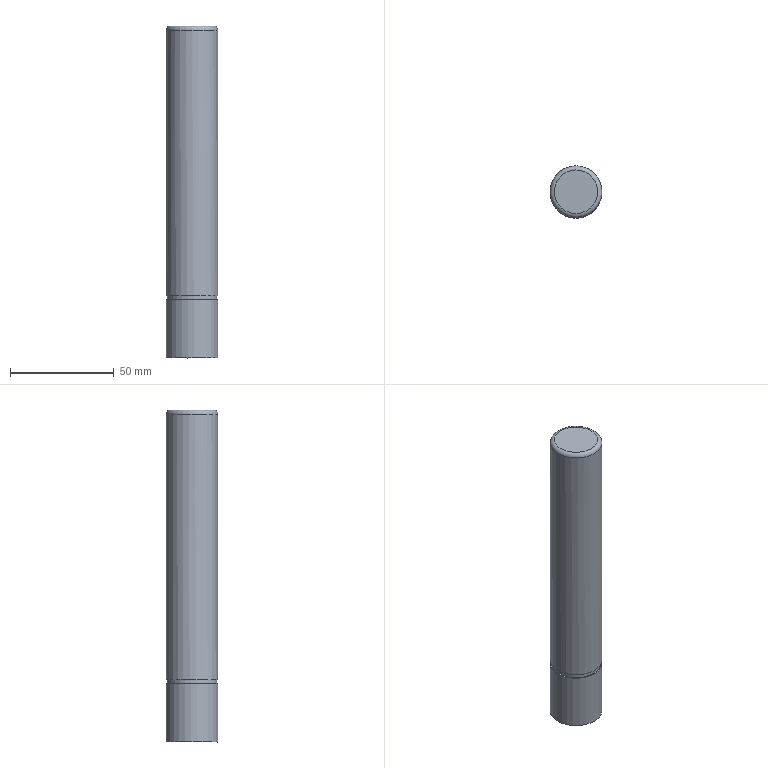Part | NX | features SGPN25-140_1 2 | 1 solid | 87 faces | box 25 x 25.002 x 160 mm | volume 77267 mm3 | plane 48 | cylinder 36 | cone 2 | torus 1 | commonest cylinder face diameters 24.8 x5 25 x3 3.389 x1 3.509 x1 4.336 x1 4.656 x1